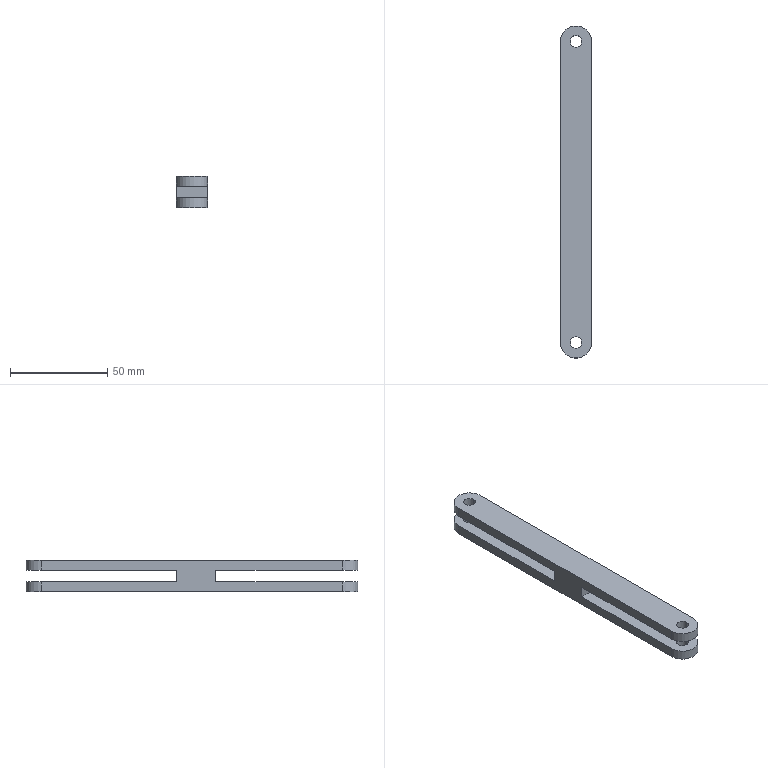Part | SolidWorks | features Extrusion 1, ICE 1 | 1 solid | 22 faces | box 16 x 171 x 16 mm | volume 28165 mm3 | cylinder 12 | plane 10 | commonest cylinder face diameters 6 x8 16 x4
STEP:
#1=CARTESIAN_POINT('',(-3.,-75.273,16.));
#2=VERTEX_POINT('',#1);
#3=CARTESIAN_POINT('',(3.,-75.273,16.));
#4=VERTEX_POINT('',#3);
#5=CARTESIAN_POINT('',(0.,-75.273,16.));
#6=DIRECTION('',(0.,0.,1.));
#7=DIRECTION('',(1.,0.,0.));
#8=AXIS2_PLACEMENT_3D('',#5,#6,#7);
#9=CIRCLE('',#8,3.);
#10=EDGE_CURVE('',#2,#4,#9,.T.);
#11=ORIENTED_EDGE('',*,*,#10,.T.);
#12=CARTESIAN_POINT('',(3.,-75.273,11.));
#13=VERTEX_POINT('',#12);
#14=CARTESIAN_POINT('',(3.,-75.273,16.));
#15=DIRECTION('',(0.,0.,-1.));
#16=VECTOR('',#15,1000.);
#17=LINE('',#14,#16);
#18=EDGE_CURVE('',#4,#13,#17,.T.);
#19=ORIENTED_EDGE('',*,*,#18,.T.);
#20=CARTESIAN_POINT('',(-3.,-75.273,11.));
#21=VERTEX_POINT('',#20);
#22=CARTESIAN_POINT('',(0.,-75.273,11.));
#23=DIRECTION('',(0.,0.,1.));
#24=DIRECTION('',(1.,0.,0.));
#25=AXIS2_PLACEMENT_3D('',#22,#23,#24);
#26=CIRCLE('',#25,3.);
#27=EDGE_CURVE('',#21,#13,#26,.T.);
#28=ORIENTED_EDGE('',*,*,#27,.F.);
#29=CARTESIAN_POINT('',(-3.,-75.273,16.));
#30=DIRECTION('',(0.,0.,-1.));
#31=VECTOR('',#30,1000.);
#32=LINE('',#29,#31);
#33=EDGE_CURVE('',#2,#21,#32,.T.);
#34=ORIENTED_EDGE('',*,*,#33,.F.);
#35=EDGE_LOOP('',(#11,#19,#28,#34));
#36=FACE_OUTER_BOUND('',#35,.T.);
#37=CARTESIAN_POINT('',(0.,-75.273,16.));
#38=DIRECTION('',(0.,0.,-1.));
#39=DIRECTION('',(-1.,0.,0.));
#40=AXIS2_PLACEMENT_3D('',#37,#38,#39);
#41=CYLINDRICAL_SURFACE('',#40,3.);
#42=ADVANCED_FACE('',(#36),#41,.F.);
#43=CARTESIAN_POINT('',(-3.,79.727,16.));
#44=VERTEX_POINT('',#43);
#45=CARTESIAN_POINT('',(3.,79.727,16.));
#46=VERTEX_POINT('',#45);
#47=CARTESIAN_POINT('',(0.,79.727,16.));
#48=DIRECTION('',(0.,0.,1.));
#49=DIRECTION('',(1.,0.,0.));
#50=AXIS2_PLACEMENT_3D('',#47,#48,#49);
#51=CIRCLE('',#50,3.);
#52=EDGE_CURVE('',#44,#46,#51,.T.);
#53=ORIENTED_EDGE('',*,*,#52,.T.);
#54=CARTESIAN_POINT('',(3.,79.727,11.));
#55=VERTEX_POINT('',#54);
#56=CARTESIAN_POINT('',(3.,79.727,16.));
#57=DIRECTION('',(0.,0.,-1.));
#58=VECTOR('',#57,1000.);
#59=LINE('',#56,#58);
#60=EDGE_CURVE('',#46,#55,#59,.T.);
#61=ORIENTED_EDGE('',*,*,#60,.T.);
#62=CARTESIAN_POINT('',(-3.,79.727,11.));
#63=VERTEX_POINT('',#62);
#64=CARTESIAN_POINT('',(0.,79.727,11.));
#65=DIRECTION('',(0.,0.,1.));
#66=DIRECTION('',(1.,0.,0.));
#67=AXIS2_PLACEMENT_3D('',#64,#65,#66);
#68=CIRCLE('',#67,3.);
#69=EDGE_CURVE('',#63,#55,#68,.T.);
#70=ORIENTED_EDGE('',*,*,#69,.F.);
#71=CARTESIAN_POINT('',(-3.,79.727,16.));
#72=DIRECTION('',(0.,0.,-1.));
#73=VECTOR('',#72,1000.);
#74=LINE('',#71,#73);
#75=EDGE_CURVE('',#44,#63,#74,.T.);
#76=ORIENTED_EDGE('',*,*,#75,.F.);
#77=EDGE_LOOP('',(#53,#61,#70,#76));
#78=FACE_OUTER_BOUND('',#77,.T.);
#79=CARTESIAN_POINT('',(0.,79.727,16.));
#80=DIRECTION('',(0.,0.,-1.));
#81=DIRECTION('',(-1.,0.,0.));
#82=AXIS2_PLACEMENT_3D('',#79,#80,#81);
#83=CYLINDRICAL_SURFACE('',#82,3.);
#84=ADVANCED_FACE('',(#78),#83,.F.);
#85=CARTESIAN_POINT('',(3.,-75.273,5.));
#86=VERTEX_POINT('',#85);
#87=CARTESIAN_POINT('',(-3.,-75.273,5.));
#88=VERTEX_POINT('',#87);
#89=CARTESIAN_POINT('',(0.,-75.273,5.));
#90=DIRECTION('',(0.,0.,-1.));
#91=DIRECTION('',(-1.,0.,0.));
#92=AXIS2_PLACEMENT_3D('',#89,#90,#91);
#93=CIRCLE('',#92,3.);
#94=EDGE_CURVE('',#86,#88,#93,.T.);
#95=ORIENTED_EDGE('',*,*,#94,.F.);
#96=CARTESIAN_POINT('',(3.,-75.273,0.));
#97=VERTEX_POINT('',#96);
#98=CARTESIAN_POINT('',(3.,-75.273,16.));
#99=DIRECTION('',(0.,0.,-1.));
#100=VECTOR('',#99,1000.);
#101=LINE('',#98,#100);
#102=EDGE_CURVE('',#86,#97,#101,.T.);
#103=ORIENTED_EDGE('',*,*,#102,.T.);
#104=CARTESIAN_POINT('',(-3.,-75.273,0.));
#105=VERTEX_POINT('',#104);
#106=CARTESIAN_POINT('',(0.,-75.273,0.));
#107=DIRECTION('',(0.,0.,1.));
#108=DIRECTION('',(1.,0.,0.));
#109=AXIS2_PLACEMENT_3D('',#106,#107,#108);
#110=CIRCLE('',#109,3.);
#111=EDGE_CURVE('',#105,#97,#110,.T.);
#112=ORIENTED_EDGE('',*,*,#111,.F.);
#113=CARTESIAN_POINT('',(-3.,-75.273,16.));
#114=DIRECTION('',(0.,0.,-1.));
#115=VECTOR('',#114,1000.);
#116=LINE('',#113,#115);
#117=EDGE_CURVE('',#88,#105,#116,.T.);
#118=ORIENTED_EDGE('',*,*,#117,.F.);
#119=EDGE_LOOP('',(#95,#103,#112,#118));
#120=FACE_OUTER_BOUND('',#119,.T.);
#121=CARTESIAN_POINT('',(0.,-75.273,16.));
#122=DIRECTION('',(0.,0.,-1.));
#123=DIRECTION('',(-1.,0.,0.));
#124=AXIS2_PLACEMENT_3D('',#121,#122,#123);
#125=CYLINDRICAL_SURFACE('',#124,3.);
#126=ADVANCED_FACE('',(#120),#125,.F.);
#127=CARTESIAN_POINT('',(3.,79.727,5.));
#128=VERTEX_POINT('',#127);
#129=CARTESIAN_POINT('',(-3.,79.727,5.));
#130=VERTEX_POINT('',#129);
#131=CARTESIAN_POINT('',(0.,79.727,5.));
#132=DIRECTION('',(0.,0.,-1.));
#133=DIRECTION('',(-1.,0.,0.));
#134=AXIS2_PLACEMENT_3D('',#131,#132,#133);
#135=CIRCLE('',#134,3.);
#136=EDGE_CURVE('',#128,#130,#135,.T.);
#137=ORIENTED_EDGE('',*,*,#136,.F.);
#138=CARTESIAN_POINT('',(3.,79.727,0.));
#139=VERTEX_POINT('',#138);
#140=CARTESIAN_POINT('',(3.,79.727,16.));
#141=DIRECTION('',(0.,0.,-1.));
#142=VECTOR('',#141,1000.);
#143=LINE('',#140,#142);
#144=EDGE_CURVE('',#128,#139,#143,.T.);
#145=ORIENTED_EDGE('',*,*,#144,.T.);
#146=CARTESIAN_POINT('',(-3.,79.727,0.));
#147=VERTEX_POINT('',#146);
#148=CARTESIAN_POINT('',(0.,79.727,0.));
#149=DIRECTION('',(0.,0.,1.));
#150=DIRECTION('',(1.,0.,0.));
#151=AXIS2_PLACEMENT_3D('',#148,#149,#150);
#152=CIRCLE('',#151,3.);
#153=EDGE_CURVE('',#147,#139,#152,.T.);
#154=ORIENTED_EDGE('',*,*,#153,.F.);
#155=CARTESIAN_POINT('',(-3.,79.727,16.));
#156=DIRECTION('',(0.,0.,-1.));
#157=VECTOR('',#156,1000.);
#158=LINE('',#155,#157);
#159=EDGE_CURVE('',#130,#147,#158,.T.);
#160=ORIENTED_EDGE('',*,*,#159,.F.);
#161=EDGE_LOOP('',(#137,#145,#154,#160));
#162=FACE_OUTER_BOUND('',#161,.T.);
#163=CARTESIAN_POINT('',(0.,79.727,16.));
#164=DIRECTION('',(0.,0.,-1.));
#165=DIRECTION('',(-1.,0.,0.));
#166=AXIS2_PLACEMENT_3D('',#163,#164,#165);
#167=CYLINDRICAL_SURFACE('',#166,3.);
#168=ADVANCED_FACE('',(#162),#167,.F.);
#169=CARTESIAN_POINT('',(-8.,79.727,5.));
#170=VERTEX_POINT('',#169);
#171=CARTESIAN_POINT('',(-8.,79.727,0.));
#172=VERTEX_POINT('',#171);
#173=CARTESIAN_POINT('',(-8.,79.727,16.));
#174=DIRECTION('',(0.,0.,-1.));
#175=VECTOR('',#174,1000.);
#176=LINE('',#173,#175);
#177=EDGE_CURVE('',#170,#172,#176,.T.);
#178=ORIENTED_EDGE('',*,*,#177,.F.);
#179=CARTESIAN_POINT('',(8.,79.727,5.));
#180=VERTEX_POINT('',#179);
#181=CARTESIAN_POINT('',(0.,79.727,5.));
#182=DIRECTION('',(0.,0.,-1.));
#183=DIRECTION('',(-1.,0.,0.));
#184=AXIS2_PLACEMENT_3D('',#181,#182,#183);
#185=CIRCLE('',#184,8.);
#186=EDGE_CURVE('',#170,#180,#185,.T.);
#187=ORIENTED_EDGE('',*,*,#186,.T.);
#188=CARTESIAN_POINT('',(8.,79.727,0.));
#189=VERTEX_POINT('',#188);
#190=CARTESIAN_POINT('',(8.,79.727,16.));
#191=DIRECTION('',(0.,0.,-1.));
#192=VECTOR('',#191,1000.);
#193=LINE('',#190,#192);
#194=EDGE_CURVE('',#180,#189,#193,.T.);
#195=ORIENTED_EDGE('',*,*,#194,.T.);
#196=CARTESIAN_POINT('',(0.,79.727,0.));
#197=DIRECTION('',(0.,0.,1.));
#198=DIRECTION('',(1.,0.,0.));
#199=AXIS2_PLACEMENT_3D('',#196,#197,#198);
#200=CIRCLE('',#199,8.);
#201=EDGE_CURVE('',#189,#172,#200,.T.);
#202=ORIENTED_EDGE('',*,*,#201,.T.);
#203=EDGE_LOOP('',(#178,#187,#195,#202));
#204=FACE_OUTER_BOUND('',#203,.T.);
#205=CARTESIAN_POINT('',(0.,79.727,16.));
#206=DIRECTION('',(0.,0.,-1.));
#207=DIRECTION('',(-1.,0.,0.));
#208=AXIS2_PLACEMENT_3D('',#205,#206,#207);
#209=CYLINDRICAL_SURFACE('',#208,8.);
#210=ADVANCED_FACE('',(#204),#209,.T.);
#211=CARTESIAN_POINT('',(8.,-75.273,5.));
#212=VERTEX_POINT('',#211);
#213=CARTESIAN_POINT('',(8.,-75.273,0.));
#214=VERTEX_POINT('',#213);
#215=CARTESIAN_POINT('',(8.,-75.273,16.));
#216=DIRECTION('',(0.,0.,-1.));
#217=VECTOR('',#216,1000.);
#218=LINE('',#215,#217);
#219=EDGE_CURVE('',#212,#214,#218,.T.);
#220=ORIENTED_EDGE('',*,*,#219,.F.);
#221=CARTESIAN_POINT('',(-8.,-75.273,5.));
#222=VERTEX_POINT('',#221);
#223=CARTESIAN_POINT('',(0.,-75.273,5.));
#224=DIRECTION('',(0.,0.,-1.));
#225=DIRECTION('',(-1.,0.,0.));
#226=AXIS2_PLACEMENT_3D('',#223,#224,#225);
#227=CIRCLE('',#226,8.);
#228=EDGE_CURVE('',#212,#222,#227,.T.);
#229=ORIENTED_EDGE('',*,*,#228,.T.);
#230=CARTESIAN_POINT('',(-8.,-75.273,0.));
#231=VERTEX_POINT('',#230);
#232=CARTESIAN_POINT('',(-8.,-75.273,16.));
#233=DIRECTION('',(0.,0.,-1.));
#234=VECTOR('',#233,1000.);
#235=LINE('',#232,#234);
#236=EDGE_CURVE('',#222,#231,#235,.T.);
#237=ORIENTED_EDGE('',*,*,#236,.T.);
#238=CARTESIAN_POINT('',(0.,-75.273,0.));
#239=DIRECTION('',(0.,0.,1.));
#240=DIRECTION('',(1.,0.,0.));
#241=AXIS2_PLACEMENT_3D('',#238,#239,#240);
#242=CIRCLE('',#241,8.);
#243=EDGE_CURVE('',#231,#214,#242,.T.);
#244=ORIENTED_EDGE('',*,*,#243,.T.);
#245=EDGE_LOOP('',(#220,#229,#237,#244));
#246=FACE_OUTER_BOUND('',#245,.T.);
#247=CARTESIAN_POINT('',(0.,-75.273,16.));
#248=DIRECTION('',(0.,0.,-1.));
#249=DIRECTION('',(-1.,0.,0.));
#250=AXIS2_PLACEMENT_3D('',#247,#248,#249);
#251=CYLINDRICAL_SURFACE('',#250,8.);
#252=ADVANCED_FACE('',(#246),#251,.T.);
#253=ORIENTED_EDGE('',*,*,#144,.F.);
#254=CARTESIAN_POINT('',(0.,79.727,5.));
#255=DIRECTION('',(0.,0.,-1.));
#256=DIRECTION('',(-1.,0.,0.));
#257=AXIS2_PLACEMENT_3D('',#254,#255,#256);
#258=CIRCLE('',#257,3.);
#259=EDGE_CURVE('',#130,#128,#258,.T.);
#260=ORIENTED_EDGE('',*,*,#259,.F.);
#261=ORIENTED_EDGE('',*,*,#159,.T.);
#262=CARTESIAN_POINT('',(0.,79.727,0.));
#263=DIRECTION('',(0.,0.,1.));
#264=DIRECTION('',(1.,0.,0.));
#265=AXIS2_PLACEMENT_3D('',#262,#263,#264);
#266=CIRCLE('',#265,3.);
#267=EDGE_CURVE('',#139,#147,#266,.T.);
#268=ORIENTED_EDGE('',*,*,#267,.F.);
#269=EDGE_LOOP('',(#253,#260,#261,#268));
#270=FACE_OUTER_BOUND('',#269,.T.);
#271=CARTESIAN_POINT('',(0.,79.727,16.));
#272=DIRECTION('',(0.,0.,-1.));
#273=DIRECTION('',(-1.,0.,0.));
#274=AXIS2_PLACEMENT_3D('',#271,#272,#273);
#275=CYLINDRICAL_SURFACE('',#274,3.);
#276=ADVANCED_FACE('',(#270),#275,.F.);
#277=ORIENTED_EDGE('',*,*,#102,.F.);
#278=CARTESIAN_POINT('',(0.,-75.273,5.));
#279=DIRECTION('',(0.,0.,-1.));
#280=DIRECTION('',(-1.,0.,0.));
#281=AXIS2_PLACEMENT_3D('',#278,#279,#280);
#282=CIRCLE('',#281,3.);
#283=EDGE_CURVE('',#88,#86,#282,.T.);
#284=ORIENTED_EDGE('',*,*,#283,.F.);
#285=ORIENTED_EDGE('',*,*,#117,.T.);
#286=CARTESIAN_POINT('',(0.,-75.273,0.));
#287=DIRECTION('',(0.,0.,1.));
#288=DIRECTION('',(1.,0.,0.));
#289=AXIS2_PLACEMENT_3D('',#286,#287,#288);
#290=CIRCLE('',#289,3.);
#291=EDGE_CURVE('',#97,#105,#290,.T.);
#292=ORIENTED_EDGE('',*,*,#291,.F.);
#293=EDGE_LOOP('',(#277,#284,#285,#292));
#294=FACE_OUTER_BOUND('',#293,.T.);
#295=CARTESIAN_POINT('',(0.,-75.273,16.));
#296=DIRECTION('',(0.,0.,-1.));
#297=DIRECTION('',(-1.,0.,0.));
#298=AXIS2_PLACEMENT_3D('',#295,#296,#297);
#299=CYLINDRICAL_SURFACE('',#298,3.);
#300=ADVANCED_FACE('',(#294),#299,.F.);
#301=ORIENTED_EDGE('',*,*,#52,.F.);
#302=CARTESIAN_POINT('',(0.,79.727,16.));
#303=DIRECTION('',(0.,0.,1.));
#304=DIRECTION('',(1.,0.,0.));
#305=AXIS2_PLACEMENT_3D('',#302,#303,#304);
#306=CIRCLE('',#305,3.);
#307=EDGE_CURVE('',#46,#44,#306,.T.);
#308=ORIENTED_EDGE('',*,*,#307,.F.);
#309=EDGE_LOOP('',(#301,#308));
#310=FACE_BOUND('',#309,.T.);
#311=CARTESIAN_POINT('',(8.,79.727,16.));
#312=VERTEX_POINT('',#311);
#313=CARTESIAN_POINT('',(-8.,79.727,16.));
#314=VERTEX_POINT('',#313);
#315=CARTESIAN_POINT('',(0.,79.727,16.));
#316=DIRECTION('',(0.,0.,1.));
#317=DIRECTION('',(1.,0.,0.));
#318=AXIS2_PLACEMENT_3D('',#315,#316,#317);
#319=CIRCLE('',#318,8.);
#320=EDGE_CURVE('',#312,#314,#319,.T.);
#321=ORIENTED_EDGE('',*,*,#320,.T.);
#322=CARTESIAN_POINT('',(-8.,-75.273,16.));
#323=VERTEX_POINT('',#322);
#324=CARTESIAN_POINT('',(-8.,79.727,16.));
#325=DIRECTION('',(0.,-1.,0.));
#326=VECTOR('',#325,1000.);
#327=LINE('',#324,#326);
#328=EDGE_CURVE('',#314,#323,#327,.T.);
#329=ORIENTED_EDGE('',*,*,#328,.T.);
#330=CARTESIAN_POINT('',(8.,-75.273,16.));
#331=VERTEX_POINT('',#330);
#332=CARTESIAN_POINT('',(0.,-75.273,16.));
#333=DIRECTION('',(0.,0.,1.));
#334=DIRECTION('',(1.,0.,0.));
#335=AXIS2_PLACEMENT_3D('',#332,#333,#334);
#336=CIRCLE('',#335,8.);
#337=EDGE_CURVE('',#323,#331,#336,.T.);
#338=ORIENTED_EDGE('',*,*,#337,.T.);
#339=CARTESIAN_POINT('',(8.,79.727,16.));
#340=DIRECTION('',(0.,1.,0.));
#341=VECTOR('',#340,1000.);
#342=LINE('',#339,#341);
#343=EDGE_CURVE('',#331,#312,#342,.T.);
#344=ORIENTED_EDGE('',*,*,#343,.T.);
#345=EDGE_LOOP('',(#321,#329,#338,#344));
#346=FACE_OUTER_BOUND('',#345,.T.);
#347=ORIENTED_EDGE('',*,*,#10,.F.);
#348=CARTESIAN_POINT('',(0.,-75.273,16.));
#349=DIRECTION('',(0.,0.,1.));
#350=DIRECTION('',(1.,0.,0.));
#351=AXIS2_PLACEMENT_3D('',#348,#349,#350);
#352=CIRCLE('',#351,3.);
#353=EDGE_CURVE('',#4,#2,#352,.T.);
#354=ORIENTED_EDGE('',*,*,#353,.F.);
#355=EDGE_LOOP('',(#347,#354));
#356=FACE_BOUND('',#355,.T.);
#357=CARTESIAN_POINT('',(0.,79.727,16.));
#358=DIRECTION('',(0.,0.,1.));
#359=DIRECTION('',(1.,0.,0.));
#360=AXIS2_PLACEMENT_3D('',#357,#358,#359);
#361=PLANE('',#360);
#362=ADVANCED_FACE('',(#310,#346,#356),#361,.T.);
#363=ORIENTED_EDGE('',*,*,#201,.F.);
#364=CARTESIAN_POINT('',(8.,79.727,0.));
#365=DIRECTION('',(0.,1.,0.));
#366=VECTOR('',#365,1000.);
#367=LINE('',#364,#366);
#368=EDGE_CURVE('',#214,#189,#367,.T.);
#369=ORIENTED_EDGE('',*,*,#368,.F.);
#370=ORIENTED_EDGE('',*,*,#243,.F.);
#371=CARTESIAN_POINT('',(-8.,79.727,0.));
#372=DIRECTION('',(0.,-1.,0.));
#373=VECTOR('',#372,1000.);
#374=LINE('',#371,#373);
#375=EDGE_CURVE('',#172,#231,#374,.T.);
#376=ORIENTED_EDGE('',*,*,#375,.F.);
#377=EDGE_LOOP('',(#363,#369,#370,#376));
#378=FACE_OUTER_BOUND('',#377,.T.);
#379=ORIENTED_EDGE('',*,*,#153,.T.);
#380=ORIENTED_EDGE('',*,*,#267,.T.);
#381=EDGE_LOOP('',(#379,#380));
#382=FACE_BOUND('',#381,.T.);
#383=ORIENTED_EDGE('',*,*,#111,.T.);
#384=ORIENTED_EDGE('',*,*,#291,.T.);
#385=EDGE_LOOP('',(#383,#384));
#386=FACE_BOUND('',#385,.T.);
#387=CARTESIAN_POINT('',(0.,79.727,0.));
#388=DIRECTION('',(0.,0.,1.));
#389=DIRECTION('',(1.,0.,0.));
#390=AXIS2_PLACEMENT_3D('',#387,#388,#389);
#391=PLANE('',#390);
#392=ADVANCED_FACE('',(#378,#382,#386),#391,.F.);
#393=CARTESIAN_POINT('',(8.,79.727,11.));
#394=VERTEX_POINT('',#393);
#395=CARTESIAN_POINT('',(8.,79.727,16.));
#396=DIRECTION('',(0.,0.,-1.));
#397=VECTOR('',#396,1000.);
#398=LINE('',#395,#397);
#399=EDGE_CURVE('',#312,#394,#398,.T.);
#400=ORIENTED_EDGE('',*,*,#399,.T.);
#401=CARTESIAN_POINT('',(-8.,79.727,11.));
#402=VERTEX_POINT('',#401);
#403=CARTESIAN_POINT('',(0.,79.727,11.));
#404=DIRECTION('',(0.,0.,1.));
#405=DIRECTION('',(1.,0.,0.));
#406=AXIS2_PLACEMENT_3D('',#403,#404,#405);
#407=CIRCLE('',#406,8.);
#408=EDGE_CURVE('',#394,#402,#407,.T.);
#409=ORIENTED_EDGE('',*,*,#408,.T.);
#410=CARTESIAN_POINT('',(-8.,79.727,16.));
#411=DIRECTION('',(0.,0.,-1.));
#412=VECTOR('',#411,1000.);
#413=LINE('',#410,#412);
#414=EDGE_CURVE('',#314,#402,#413,.T.);
#415=ORIENTED_EDGE('',*,*,#414,.F.);
#416=ORIENTED_EDGE('',*,*,#320,.F.);
#417=EDGE_LOOP('',(#400,#409,#415,#416));
#418=FACE_OUTER_BOUND('',#417,.T.);
#419=CARTESIAN_POINT('',(0.,79.727,16.));
#420=DIRECTION('',(0.,0.,-1.));
#421=DIRECTION('',(-1.,0.,0.));
#422=AXIS2_PLACEMENT_3D('',#419,#420,#421);
#423=CYLINDRICAL_SURFACE('',#422,8.);
#424=ADVANCED_FACE('',(#418),#423,.T.);
#425=CARTESIAN_POINT('',(-8.,10.,11.));
#426=VERTEX_POINT('',#425);
#427=CARTESIAN_POINT('',(-8.,10.,5.));
#428=VERTEX_POINT('',#427);
#429=CARTESIAN_POINT('',(-8.,10.,11.));
#430=DIRECTION('',(0.,0.,-1.));
#431=VECTOR('',#430,1000.);
#432=LINE('',#429,#431);
#433=EDGE_CURVE('',#426,#428,#432,.T.);
#434=ORIENTED_EDGE('',*,*,#433,.T.);
#435=CARTESIAN_POINT('',(-8.,149.453,5.));
#436=DIRECTION('',(0.,1.,0.));
#437=VECTOR('',#436,1000.);
#438=LINE('',#435,#437);
#439=EDGE_CURVE('',#428,#170,#438,.T.);
#440=ORIENTED_EDGE('',*,*,#439,.T.);
#441=ORIENTED_EDGE('',*,*,#177,.T.);
#442=ORIENTED_EDGE('',*,*,#375,.T.);
#443=ORIENTED_EDGE('',*,*,#236,.F.);
#444=CARTESIAN_POINT('',(-8.,-10.,5.));
#445=VERTEX_POINT('',#444);
#446=CARTESIAN_POINT('',(-8.,-156.547,5.));
#447=DIRECTION('',(0.,1.,0.));
#448=VECTOR('',#447,1000.);
#449=LINE('',#446,#448);
#450=EDGE_CURVE('',#222,#445,#449,.T.);
#451=ORIENTED_EDGE('',*,*,#450,.T.);
#452=CARTESIAN_POINT('',(-8.,-10.,11.));
#453=VERTEX_POINT('',#452);
#454=CARTESIAN_POINT('',(-8.,-10.,11.));
#455=DIRECTION('',(0.,0.,1.));
#456=VECTOR('',#455,1000.);
#457=LINE('',#454,#456);
#458=EDGE_CURVE('',#445,#453,#457,.T.);
#459=ORIENTED_EDGE('',*,*,#458,.T.);
#460=CARTESIAN_POINT('',(-8.,-75.273,11.));
#461=VERTEX_POINT('',#460);
#462=CARTESIAN_POINT('',(-8.,-156.547,11.));
#463=DIRECTION('',(0.,-1.,0.));
#464=VECTOR('',#463,1000.);
#465=LINE('',#462,#464);
#466=EDGE_CURVE('',#453,#461,#465,.T.);
#467=ORIENTED_EDGE('',*,*,#466,.T.);
#468=CARTESIAN_POINT('',(-8.,-75.273,16.));
#469=DIRECTION('',(0.,0.,-1.));
#470=VECTOR('',#469,1000.);
#471=LINE('',#468,#470);
#472=EDGE_CURVE('',#323,#461,#471,.T.);
#473=ORIENTED_EDGE('',*,*,#472,.F.);
#474=ORIENTED_EDGE('',*,*,#328,.F.);
#475=ORIENTED_EDGE('',*,*,#414,.T.);
#476=CARTESIAN_POINT('',(-8.,149.453,11.));
#477=DIRECTION('',(0.,-1.,0.));
#478=VECTOR('',#477,1000.);
#479=LINE('',#476,#478);
#480=EDGE_CURVE('',#402,#426,#479,.T.);
#481=ORIENTED_EDGE('',*,*,#480,.T.);
#482=EDGE_LOOP('',(#434,#440,#441,#442,#443,#451,#459,#467,#473,#474,#475,#481));
#483=FACE_OUTER_BOUND('',#482,.T.);
#484=CARTESIAN_POINT('',(-8.,79.727,16.));
#485=DIRECTION('',(1.,0.,0.));
#486=DIRECTION('',(0.,1.,0.));
#487=AXIS2_PLACEMENT_3D('',#484,#485,#486);
#488=PLANE('',#487);
#489=ADVANCED_FACE('',(#483),#488,.F.);
#490=ORIENTED_EDGE('',*,*,#472,.T.);
#491=CARTESIAN_POINT('',(8.,-75.273,11.));
#492=VERTEX_POINT('',#491);
#493=CARTESIAN_POINT('',(0.,-75.273,11.));
#494=DIRECTION('',(0.,0.,1.));
#495=DIRECTION('',(1.,0.,0.));
#496=AXIS2_PLACEMENT_3D('',#493,#494,#495);
#497=CIRCLE('',#496,8.);
#498=EDGE_CURVE('',#461,#492,#497,.T.);
#499=ORIENTED_EDGE('',*,*,#498,.T.);
#500=CARTESIAN_POINT('',(8.,-75.273,16.));
#501=DIRECTION('',(0.,0.,-1.));
#502=VECTOR('',#501,1000.);
#503=LINE('',#500,#502);
#504=EDGE_CURVE('',#331,#492,#503,.T.);
#505=ORIENTED_EDGE('',*,*,#504,.F.);
#506=ORIENTED_EDGE('',*,*,#337,.F.);
#507=EDGE_LOOP('',(#490,#499,#505,#506));
#508=FACE_OUTER_BOUND('',#507,.T.);
#509=CARTESIAN_POINT('',(0.,-75.273,16.));
#510=DIRECTION('',(0.,0.,-1.));
#511=DIRECTION('',(-1.,0.,0.));
#512=AXIS2_PLACEMENT_3D('',#509,#510,#511);
#513=CYLINDRICAL_SURFACE('',#512,8.);
#514=ADVANCED_FACE('',(#508),#513,.T.);
#515=ORIENTED_EDGE('',*,*,#194,.F.);
#516=CARTESIAN_POINT('',(8.,10.,5.));
#517=VERTEX_POINT('',#516);
#518=CARTESIAN_POINT('',(8.,149.453,5.));
#519=DIRECTION('',(0.,1.,0.));
#520=VECTOR('',#519,1000.);
#521=LINE('',#518,#520);
#522=EDGE_CURVE('',#517,#180,#521,.T.);
#523=ORIENTED_EDGE('',*,*,#522,.F.);
#524=CARTESIAN_POINT('',(8.,10.,11.));
#525=VERTEX_POINT('',#524);
#526=CARTESIAN_POINT('',(8.,10.,11.));
#527=DIRECTION('',(0.,0.,-1.));
#528=VECTOR('',#527,1000.);
#529=LINE('',#526,#528);
#530=EDGE_CURVE('',#525,#517,#529,.T.);
#531=ORIENTED_EDGE('',*,*,#530,.F.);
#532=CARTESIAN_POINT('',(8.,149.453,11.));
#533=DIRECTION('',(0.,-1.,0.));
#534=VECTOR('',#533,1000.);
#535=LINE('',#532,#534);
#536=EDGE_CURVE('',#394,#525,#535,.T.);
#537=ORIENTED_EDGE('',*,*,#536,.F.);
#538=ORIENTED_EDGE('',*,*,#399,.F.);
#539=ORIENTED_EDGE('',*,*,#343,.F.);
#540=ORIENTED_EDGE('',*,*,#504,.T.);
#541=CARTESIAN_POINT('',(8.,-10.,11.));
#542=VERTEX_POINT('',#541);
#543=CARTESIAN_POINT('',(8.,-156.547,11.));
#544=DIRECTION('',(0.,-1.,0.));
#545=VECTOR('',#544,1000.);
#546=LINE('',#543,#545);
#547=EDGE_CURVE('',#542,#492,#546,.T.);
#548=ORIENTED_EDGE('',*,*,#547,.F.);
#549=CARTESIAN_POINT('',(8.,-10.,5.));
#550=VERTEX_POINT('',#549);
#551=CARTESIAN_POINT('',(8.,-10.,11.));
#552=DIRECTION('',(0.,0.,1.));
#553=VECTOR('',#552,1000.);
#554=LINE('',#551,#553);
#555=EDGE_CURVE('',#550,#542,#554,.T.);
#556=ORIENTED_EDGE('',*,*,#555,.F.);
#557=CARTESIAN_POINT('',(8.,-156.547,5.));
#558=DIRECTION('',(0.,1.,0.));
#559=VECTOR('',#558,1000.);
#560=LINE('',#557,#559);
#561=EDGE_CURVE('',#212,#550,#560,.T.);
#562=ORIENTED_EDGE('',*,*,#561,.F.);
#563=ORIENTED_EDGE('',*,*,#219,.T.);
#564=ORIENTED_EDGE('',*,*,#368,.T.);
#565=EDGE_LOOP('',(#515,#523,#531,#537,#538,#539,#540,#548,#556,#562,#563,#564));
#566=FACE_OUTER_BOUND('',#565,.T.);
#567=CARTESIAN_POINT('',(8.,79.727,16.));
#568=DIRECTION('',(-1.,0.,0.));
#569=DIRECTION('',(0.,-1.,0.));
#570=AXIS2_PLACEMENT_3D('',#567,#568,#569);
#571=PLANE('',#570);
#572=ADVANCED_FACE('',(#566),#571,.F.);
#573=ORIENTED_EDGE('',*,*,#60,.F.);
#574=ORIENTED_EDGE('',*,*,#307,.T.);
#575=ORIENTED_EDGE('',*,*,#75,.T.);
#576=CARTESIAN_POINT('',(0.,79.727,11.));
#577=DIRECTION('',(0.,0.,1.));
#578=DIRECTION('',(1.,0.,0.));
#579=AXIS2_PLACEMENT_3D('',#576,#577,#578);
#580=CIRCLE('',#579,3.);
#581=EDGE_CURVE('',#55,#63,#580,.T.);
#582=ORIENTED_EDGE('',*,*,#581,.F.);
#583=EDGE_LOOP('',(#573,#574,#575,#582));
#584=FACE_OUTER_BOUND('',#583,.T.);
#585=CARTESIAN_POINT('',(0.,79.727,16.));
#586=DIRECTION('',(0.,0.,-1.));
#587=DIRECTION('',(-1.,0.,0.));
#588=AXIS2_PLACEMENT_3D('',#585,#586,#587);
#589=CYLINDRICAL_SURFACE('',#588,3.);
#590=ADVANCED_FACE('',(#584),#589,.F.);
#591=ORIENTED_EDGE('',*,*,#18,.F.);
#592=ORIENTED_EDGE('',*,*,#353,.T.);
#593=ORIENTED_EDGE('',*,*,#33,.T.);
#594=CARTESIAN_POINT('',(0.,-75.273,11.));
#595=DIRECTION('',(0.,0.,1.));
#596=DIRECTION('',(1.,0.,0.));
#597=AXIS2_PLACEMENT_3D('',#594,#595,#596);
#598=CIRCLE('',#597,3.);
#599=EDGE_CURVE('',#13,#21,#598,.T.);
#600=ORIENTED_EDGE('',*,*,#599,.F.);
#601=EDGE_LOOP('',(#591,#592,#593,#600));
#602=FACE_OUTER_BOUND('',#601,.T.);
#603=CARTESIAN_POINT('',(0.,-75.273,16.));
#604=DIRECTION('',(0.,0.,-1.));
#605=DIRECTION('',(-1.,0.,0.));
#606=AXIS2_PLACEMENT_3D('',#603,#604,#605);
#607=CYLINDRICAL_SURFACE('',#606,3.);
#608=ADVANCED_FACE('',(#602),#607,.F.);
#609=ORIENTED_EDGE('',*,*,#283,.T.);
#610=ORIENTED_EDGE('',*,*,#94,.T.);
#611=EDGE_LOOP('',(#609,#610));
#612=FACE_BOUND('',#611,.T.);
#613=ORIENTED_EDGE('',*,*,#561,.T.);
#614=CARTESIAN_POINT('',(-8.,-10.,5.));
#615=DIRECTION('',(1.,0.,0.));
#616=VECTOR('',#615,1000.);
#617=LINE('',#614,#616);
#618=EDGE_CURVE('',#445,#550,#617,.T.);
#619=ORIENTED_EDGE('',*,*,#618,.F.);
#620=ORIENTED_EDGE('',*,*,#450,.F.);
#621=ORIENTED_EDGE('',*,*,#228,.F.);
#622=EDGE_LOOP('',(#613,#619,#620,#621));
#623=FACE_OUTER_BOUND('',#622,.T.);
#624=CARTESIAN_POINT('',(-8.,-156.547,5.));
#625=DIRECTION('',(0.,0.,-1.));
#626=DIRECTION('',(-1.,0.,0.));
#627=AXIS2_PLACEMENT_3D('',#624,#625,#626);
#628=PLANE('',#627);
#629=ADVANCED_FACE('',(#612,#623),#628,.F.);
#630=ORIENTED_EDGE('',*,*,#27,.T.);
#631=ORIENTED_EDGE('',*,*,#599,.T.);
#632=EDGE_LOOP('',(#630,#631));
#633=FACE_BOUND('',#632,.T.);
#634=ORIENTED_EDGE('',*,*,#466,.F.);
#635=CARTESIAN_POINT('',(-8.,-10.,11.));
#636=DIRECTION('',(1.,0.,0.));
#637=VECTOR('',#636,1000.);
#638=LINE('',#635,#637);
#639=EDGE_CURVE('',#453,#542,#638,.T.);
#640=ORIENTED_EDGE('',*,*,#639,.T.);
#641=ORIENTED_EDGE('',*,*,#547,.T.);
#642=ORIENTED_EDGE('',*,*,#498,.F.);
#643=EDGE_LOOP('',(#634,#640,#641,#642));
#644=FACE_OUTER_BOUND('',#643,.T.);
#645=CARTESIAN_POINT('',(-8.,-156.547,11.));
#646=DIRECTION('',(0.,0.,1.));
#647=DIRECTION('',(1.,0.,0.));
#648=AXIS2_PLACEMENT_3D('',#645,#646,#647);
#649=PLANE('',#648);
#650=ADVANCED_FACE('',(#633,#644),#649,.F.);
#651=ORIENTED_EDGE('',*,*,#555,.T.);
#652=ORIENTED_EDGE('',*,*,#639,.F.);
#653=ORIENTED_EDGE('',*,*,#458,.F.);
#654=ORIENTED_EDGE('',*,*,#618,.T.);
#655=EDGE_LOOP('',(#651,#652,#653,#654));
#656=FACE_OUTER_BOUND('',#655,.T.);
#657=CARTESIAN_POINT('',(-8.,-10.,11.));
#658=DIRECTION('',(0.,1.,0.));
#659=DIRECTION('',(-1.,0.,0.));
#660=AXIS2_PLACEMENT_3D('',#657,#658,#659);
#661=PLANE('',#660);
#662=ADVANCED_FACE('',(#656),#661,.F.);
#663=ORIENTED_EDGE('',*,*,#259,.T.);
#664=ORIENTED_EDGE('',*,*,#136,.T.);
#665=EDGE_LOOP('',(#663,#664));
#666=FACE_BOUND('',#665,.T.);
#667=ORIENTED_EDGE('',*,*,#439,.F.);
#668=CARTESIAN_POINT('',(-8.,10.,5.));
#669=DIRECTION('',(1.,0.,0.));
#670=VECTOR('',#669,1000.);
#671=LINE('',#668,#670);
#672=EDGE_CURVE('',#428,#517,#671,.T.);
#673=ORIENTED_EDGE('',*,*,#672,.T.);
#674=ORIENTED_EDGE('',*,*,#522,.T.);
#675=ORIENTED_EDGE('',*,*,#186,.F.);
#676=EDGE_LOOP('',(#667,#673,#674,#675));
#677=FACE_OUTER_BOUND('',#676,.T.);
#678=CARTESIAN_POINT('',(-8.,149.453,5.));
#679=DIRECTION('',(0.,0.,-1.));
#680=DIRECTION('',(-1.,0.,0.));
#681=AXIS2_PLACEMENT_3D('',#678,#679,#680);
#682=PLANE('',#681);
#683=ADVANCED_FACE('',(#666,#677),#682,.F.);
#684=ORIENTED_EDGE('',*,*,#69,.T.);
#685=ORIENTED_EDGE('',*,*,#581,.T.);
#686=EDGE_LOOP('',(#684,#685));
#687=FACE_BOUND('',#686,.T.);
#688=ORIENTED_EDGE('',*,*,#536,.T.);
#689=CARTESIAN_POINT('',(-8.,10.,11.));
#690=DIRECTION('',(1.,0.,0.));
#691=VECTOR('',#690,1000.);
#692=LINE('',#689,#691);
#693=EDGE_CURVE('',#426,#525,#692,.T.);
#694=ORIENTED_EDGE('',*,*,#693,.F.);
#695=ORIENTED_EDGE('',*,*,#480,.F.);
#696=ORIENTED_EDGE('',*,*,#408,.F.);
#697=EDGE_LOOP('',(#688,#694,#695,#696));
#698=FACE_OUTER_BOUND('',#697,.T.);
#699=CARTESIAN_POINT('',(-8.,149.453,11.));
#700=DIRECTION('',(0.,0.,1.));
#701=DIRECTION('',(1.,0.,0.));
#702=AXIS2_PLACEMENT_3D('',#699,#700,#701);
#703=PLANE('',#702);
#704=ADVANCED_FACE('',(#687,#698),#703,.F.);
#705=ORIENTED_EDGE('',*,*,#530,.T.);
#706=ORIENTED_EDGE('',*,*,#672,.F.);
#707=ORIENTED_EDGE('',*,*,#433,.F.);
#708=ORIENTED_EDGE('',*,*,#693,.T.);
#709=EDGE_LOOP('',(#705,#706,#707,#708));
#710=FACE_OUTER_BOUND('',#709,.T.);
#711=CARTESIAN_POINT('',(-8.,10.,11.));
#712=DIRECTION('',(0.,-1.,0.));
#713=DIRECTION('',(1.,0.,0.));
#714=AXIS2_PLACEMENT_3D('',#711,#712,#713);
#715=PLANE('',#714);
#716=ADVANCED_FACE('',(#710),#715,.F.);
#717=CLOSED_SHELL('',(#42,#84,#126,#168,#210,#252,#276,#300,#362,#392,#424,#489,#514,#572,#590,#608,#629,#650,#662,#683,#704,#716));
#718=MANIFOLD_SOLID_BREP('',#717);
#719=CARTESIAN_POINT('',(0.,0.,0.));
#720=DIRECTION('',(0.,0.,1.));
#721=DIRECTION('',(1.,0.,0.));
#722=AXIS2_PLACEMENT_3D('',#719,#720,#721);
#723=(LENGTH_UNIT()NAMED_UNIT(*)SI_UNIT(.MILLI.,.METRE.));
#724=UNCERTAINTY_MEASURE_WITH_UNIT(LENGTH_MEASURE(0.00001),#723,'','');
#725=(NAMED_UNIT(*)PLANE_ANGLE_UNIT()SI_UNIT($,.RADIAN.));
#726=(NAMED_UNIT(*)SI_UNIT($,.STERADIAN.)SOLID_ANGLE_UNIT());
#727=(GEOMETRIC_REPRESENTATION_CONTEXT(3)GLOBAL_UNCERTAINTY_ASSIGNED_CONTEXT((#724))GLOBAL_UNIT_ASSIGNED_CONTEXT((#723,#725,#726))REPRESENTATION_CONTEXT('',''));
#728=ADVANCED_BREP_SHAPE_REPRESENTATION('',(#718,#722),#727);